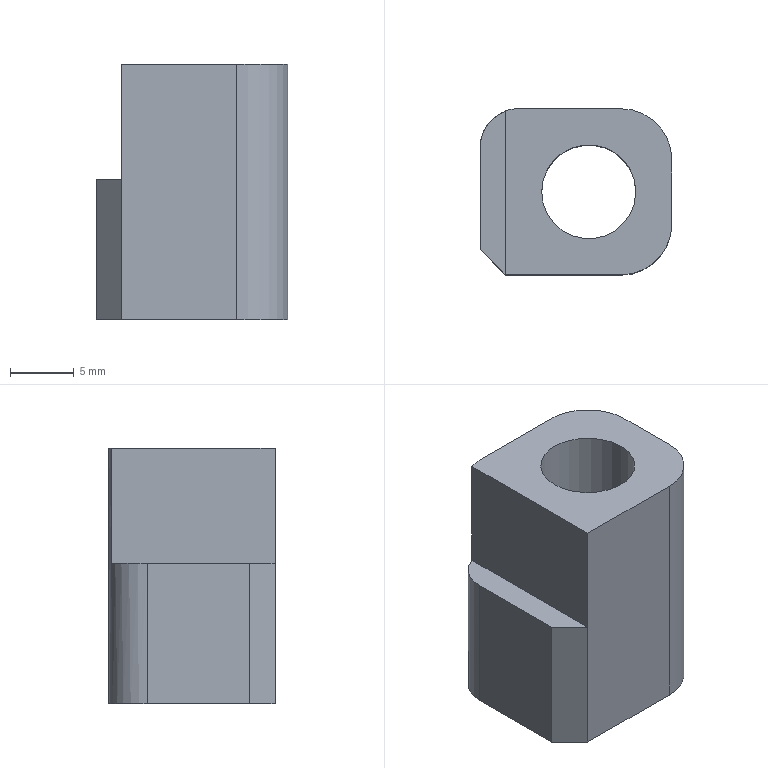Part | STEP file | 1 solid | 13 faces | box 15 x 13 x 20 mm | volume 2634 mm3 | plane 9 | cylinder 4 | commonest cylinder face diameters 8 x2 6 x1 7.36 x1
STEP:
#1=CARTESIAN_POINT('',(272.5,-10.,-2.));
#2=VERTEX_POINT('',#1);
#3=CARTESIAN_POINT('',(272.5,-15.,-2.));
#4=VERTEX_POINT('',#3);
#5=CARTESIAN_POINT('',(272.5,-12.5,-2.));
#6=DIRECTION('',(0.,-1.,0.));
#7=VECTOR('',#6,1.);
#8=LINE('',#5,#7);
#9=EDGE_CURVE('',#2,#4,#8,.T.);
#10=ORIENTED_EDGE('',*,*,#9,.F.);
#11=CARTESIAN_POINT('',(268.5,-6.,-2.));
#12=VERTEX_POINT('',#11);
#13=CARTESIAN_POINT('',(268.5,-10.,-2.));
#14=DIRECTION('',(0.,0.,1.));
#15=DIRECTION('',(1.,0.,0.));
#16=AXIS2_PLACEMENT_3D('',#13,#14,#15);
#17=CIRCLE('',#16,4.);
#18=EDGE_CURVE('',#2,#12,#17,.T.);
#19=ORIENTED_EDGE('',*,*,#18,.T.);
#20=CARTESIAN_POINT('',(260.5,-6.,-2.));
#21=VERTEX_POINT('',#20);
#22=CARTESIAN_POINT('',(266.,-6.,-2.));
#23=DIRECTION('',(1.,0.,0.));
#24=VECTOR('',#23,1.);
#25=LINE('',#22,#24);
#26=EDGE_CURVE('',#21,#12,#25,.T.);
#27=ORIENTED_EDGE('',*,*,#26,.F.);
#28=CARTESIAN_POINT('',(259.5,-6.172,-2.));
#29=VERTEX_POINT('',#28);
#30=CARTESIAN_POINT('',(260.5,-9.,-2.));
#31=DIRECTION('',(0.,0.,1.));
#32=DIRECTION('',(1.,0.,0.));
#33=AXIS2_PLACEMENT_3D('',#30,#31,#32);
#34=CIRCLE('',#33,3.);
#35=EDGE_CURVE('',#21,#29,#34,.T.);
#36=ORIENTED_EDGE('',*,*,#35,.T.);
#37=CARTESIAN_POINT('',(259.5,-19.,-2.));
#38=VERTEX_POINT('',#37);
#39=CARTESIAN_POINT('',(259.5,-12.5,-2.));
#40=DIRECTION('',(0.,1.,0.));
#41=VECTOR('',#40,1.);
#42=LINE('',#39,#41);
#43=EDGE_CURVE('',#38,#29,#42,.T.);
#44=ORIENTED_EDGE('',*,*,#43,.F.);
#45=CARTESIAN_POINT('',(268.5,-19.,-2.));
#46=VERTEX_POINT('',#45);
#47=CARTESIAN_POINT('',(266.,-19.,-2.));
#48=DIRECTION('',(-1.,0.,0.));
#49=VECTOR('',#48,1.);
#50=LINE('',#47,#49);
#51=EDGE_CURVE('',#46,#38,#50,.T.);
#52=ORIENTED_EDGE('',*,*,#51,.F.);
#53=CARTESIAN_POINT('',(268.5,-15.,-2.));
#54=DIRECTION('',(0.,0.,1.));
#55=DIRECTION('',(1.,0.,0.));
#56=AXIS2_PLACEMENT_3D('',#53,#54,#55);
#57=CIRCLE('',#56,4.);
#58=EDGE_CURVE('',#46,#4,#57,.T.);
#59=ORIENTED_EDGE('',*,*,#58,.T.);
#60=EDGE_LOOP('',(#10,#19,#27,#36,#44,#52,#59));
#61=FACE_BOUND('',#60,.T.);
#62=CARTESIAN_POINT('',(269.68,-12.5,-2.));
#63=VERTEX_POINT('',#62);
#64=CARTESIAN_POINT('',(266.,-12.5,-2.));
#65=DIRECTION('',(0.,0.,-1.));
#66=DIRECTION('',(1.,0.,0.));
#67=AXIS2_PLACEMENT_3D('',#64,#65,#66);
#68=CIRCLE('',#67,3.68);
#69=EDGE_CURVE('',#63,#63,#68,.T.);
#70=ORIENTED_EDGE('',*,*,#69,.T.);
#71=EDGE_LOOP('',(#70));
#72=FACE_BOUND('',#71,.T.);
#73=CARTESIAN_POINT('',(266.,-12.5,-2.));
#74=DIRECTION('',(0.,0.,1.));
#75=DIRECTION('',(1.,0.,0.));
#76=AXIS2_PLACEMENT_3D('',#73,#74,#75);
#77=PLANE('',#76);
#78=ADVANCED_FACE('',(#61,#72),#77,.T.);
#79=CARTESIAN_POINT('',(259.5,-19.,-11.));
#80=VERTEX_POINT('',#79);
#81=CARTESIAN_POINT('',(259.5,-19.,-22.));
#82=DIRECTION('',(0.,0.,1.));
#83=VECTOR('',#82,1.);
#84=LINE('',#81,#83);
#85=EDGE_CURVE('',#80,#38,#84,.T.);
#86=ORIENTED_EDGE('',*,*,#85,.F.);
#87=CARTESIAN_POINT('',(259.5,-19.,-22.));
#88=VERTEX_POINT('',#87);
#89=CARTESIAN_POINT('',(259.5,-19.,-22.));
#90=DIRECTION('',(0.,0.,-1.));
#91=VECTOR('',#90,1.);
#92=LINE('',#89,#91);
#93=EDGE_CURVE('',#80,#88,#92,.T.);
#94=ORIENTED_EDGE('',*,*,#93,.T.);
#95=CARTESIAN_POINT('',(268.5,-19.,-22.));
#96=VERTEX_POINT('',#95);
#97=CARTESIAN_POINT('',(266.,-19.,-22.));
#98=DIRECTION('',(1.,0.,0.));
#99=VECTOR('',#98,1.);
#100=LINE('',#97,#99);
#101=EDGE_CURVE('',#88,#96,#100,.T.);
#102=ORIENTED_EDGE('',*,*,#101,.T.);
#103=CARTESIAN_POINT('',(268.5,-19.,-22.));
#104=DIRECTION('',(0.,0.,1.));
#105=VECTOR('',#104,1.);
#106=LINE('',#103,#105);
#107=EDGE_CURVE('',#96,#46,#106,.T.);
#108=ORIENTED_EDGE('',*,*,#107,.T.);
#109=ORIENTED_EDGE('',*,*,#51,.T.);
#110=EDGE_LOOP('',(#86,#94,#102,#108,#109));
#111=FACE_OUTER_BOUND('',#110,.T.);
#112=CARTESIAN_POINT('',(266.,-19.,-22.));
#113=DIRECTION('',(0.,-1.,0.));
#114=DIRECTION('',(0.,0.,-1.));
#115=AXIS2_PLACEMENT_3D('',#112,#113,#114);
#116=PLANE('',#115);
#117=ADVANCED_FACE('',(#111),#116,.T.);
#118=ORIENTED_EDGE('',*,*,#43,.T.);
#119=CARTESIAN_POINT('',(259.5,-6.172,-11.));
#120=VERTEX_POINT('',#119);
#121=CARTESIAN_POINT('',(259.5,-6.172,-2.));
#122=DIRECTION('',(0.,0.,-1.));
#123=VECTOR('',#122,1.);
#124=LINE('',#121,#123);
#125=EDGE_CURVE('',#29,#120,#124,.T.);
#126=ORIENTED_EDGE('',*,*,#125,.T.);
#127=CARTESIAN_POINT('',(259.5,-12.5,-11.));
#128=DIRECTION('',(0.,1.,0.));
#129=VECTOR('',#128,1.);
#130=LINE('',#127,#129);
#131=EDGE_CURVE('',#80,#120,#130,.T.);
#132=ORIENTED_EDGE('',*,*,#131,.F.);
#133=ORIENTED_EDGE('',*,*,#85,.T.);
#134=EDGE_LOOP('',(#118,#126,#132,#133));
#135=FACE_OUTER_BOUND('',#134,.T.);
#136=CARTESIAN_POINT('',(259.5,-12.5,-22.));
#137=DIRECTION('',(-1.,0.,0.));
#138=DIRECTION('',(0.,0.,1.));
#139=AXIS2_PLACEMENT_3D('',#136,#137,#138);
#140=PLANE('',#139);
#141=ADVANCED_FACE('',(#135),#140,.T.);
#142=ORIENTED_EDGE('',*,*,#26,.T.);
#143=CARTESIAN_POINT('',(268.5,-6.,-22.));
#144=VERTEX_POINT('',#143);
#145=CARTESIAN_POINT('',(268.5,-6.,-22.));
#146=DIRECTION('',(0.,0.,-1.));
#147=VECTOR('',#146,1.);
#148=LINE('',#145,#147);
#149=EDGE_CURVE('',#12,#144,#148,.T.);
#150=ORIENTED_EDGE('',*,*,#149,.T.);
#151=CARTESIAN_POINT('',(260.5,-6.,-22.));
#152=VERTEX_POINT('',#151);
#153=CARTESIAN_POINT('',(266.,-6.,-22.));
#154=DIRECTION('',(-1.,0.,0.));
#155=VECTOR('',#154,1.);
#156=LINE('',#153,#155);
#157=EDGE_CURVE('',#144,#152,#156,.T.);
#158=ORIENTED_EDGE('',*,*,#157,.T.);
#159=CARTESIAN_POINT('',(260.5,-6.,-22.));
#160=DIRECTION('',(0.,0.,1.));
#161=VECTOR('',#160,1.);
#162=LINE('',#159,#161);
#163=EDGE_CURVE('',#152,#21,#162,.T.);
#164=ORIENTED_EDGE('',*,*,#163,.T.);
#165=EDGE_LOOP('',(#142,#150,#158,#164));
#166=FACE_OUTER_BOUND('',#165,.T.);
#167=CARTESIAN_POINT('',(266.,-6.,-22.));
#168=DIRECTION('',(0.,1.,0.));
#169=DIRECTION('',(0.,0.,1.));
#170=AXIS2_PLACEMENT_3D('',#167,#168,#169);
#171=PLANE('',#170);
#172=ADVANCED_FACE('',(#166),#171,.T.);
#173=ORIENTED_EDGE('',*,*,#101,.F.);
#174=CARTESIAN_POINT('',(257.5,-17.,-22.));
#175=VERTEX_POINT('',#174);
#176=CARTESIAN_POINT('',(259.5,-19.,-22.));
#177=DIRECTION('',(-0.7071,0.7071,0.));
#178=VECTOR('',#177,1.);
#179=LINE('',#176,#178);
#180=EDGE_CURVE('',#88,#175,#179,.T.);
#181=ORIENTED_EDGE('',*,*,#180,.T.);
#182=CARTESIAN_POINT('',(257.5,-9.,-22.));
#183=VERTEX_POINT('',#182);
#184=CARTESIAN_POINT('',(257.5,-12.5,-22.));
#185=DIRECTION('',(0.,-1.,0.));
#186=VECTOR('',#185,1.);
#187=LINE('',#184,#186);
#188=EDGE_CURVE('',#183,#175,#187,.T.);
#189=ORIENTED_EDGE('',*,*,#188,.F.);
#190=CARTESIAN_POINT('',(260.5,-9.,-22.));
#191=DIRECTION('',(0.,0.,-1.));
#192=DIRECTION('',(-1.,0.,0.));
#193=AXIS2_PLACEMENT_3D('',#190,#191,#192);
#194=CIRCLE('',#193,3.);
#195=EDGE_CURVE('',#183,#152,#194,.T.);
#196=ORIENTED_EDGE('',*,*,#195,.T.);
#197=ORIENTED_EDGE('',*,*,#157,.F.);
#198=CARTESIAN_POINT('',(272.5,-10.,-22.));
#199=VERTEX_POINT('',#198);
#200=CARTESIAN_POINT('',(268.5,-10.,-22.));
#201=DIRECTION('',(0.,0.,-1.));
#202=DIRECTION('',(-1.,0.,0.));
#203=AXIS2_PLACEMENT_3D('',#200,#201,#202);
#204=CIRCLE('',#203,4.);
#205=EDGE_CURVE('',#144,#199,#204,.T.);
#206=ORIENTED_EDGE('',*,*,#205,.T.);
#207=CARTESIAN_POINT('',(272.5,-15.,-22.));
#208=VERTEX_POINT('',#207);
#209=CARTESIAN_POINT('',(272.5,-12.5,-22.));
#210=DIRECTION('',(0.,1.,0.));
#211=VECTOR('',#210,1.);
#212=LINE('',#209,#211);
#213=EDGE_CURVE('',#208,#199,#212,.T.);
#214=ORIENTED_EDGE('',*,*,#213,.F.);
#215=CARTESIAN_POINT('',(268.5,-15.,-22.));
#216=DIRECTION('',(0.,0.,-1.));
#217=DIRECTION('',(-1.,0.,0.));
#218=AXIS2_PLACEMENT_3D('',#215,#216,#217);
#219=CIRCLE('',#218,4.);
#220=EDGE_CURVE('',#208,#96,#219,.T.);
#221=ORIENTED_EDGE('',*,*,#220,.T.);
#222=EDGE_LOOP('',(#173,#181,#189,#196,#197,#206,#214,#221));
#223=FACE_BOUND('',#222,.T.);
#224=CARTESIAN_POINT('',(262.32,-12.5,-22.));
#225=VERTEX_POINT('',#224);
#226=CARTESIAN_POINT('',(266.,-12.5,-22.));
#227=DIRECTION('',(0.,0.,-1.));
#228=DIRECTION('',(-1.,0.,0.));
#229=AXIS2_PLACEMENT_3D('',#226,#227,#228);
#230=CIRCLE('',#229,3.68);
#231=EDGE_CURVE('',#225,#225,#230,.T.);
#232=ORIENTED_EDGE('',*,*,#231,.F.);
#233=EDGE_LOOP('',(#232));
#234=FACE_BOUND('',#233,.T.);
#235=CARTESIAN_POINT('',(266.,-12.5,-22.));
#236=DIRECTION('',(0.,0.,-1.));
#237=DIRECTION('',(-1.,0.,0.));
#238=AXIS2_PLACEMENT_3D('',#235,#236,#237);
#239=PLANE('',#238);
#240=ADVANCED_FACE('',(#223,#234),#239,.T.);
#241=ORIENTED_EDGE('',*,*,#213,.T.);
#242=CARTESIAN_POINT('',(272.5,-10.,-22.));
#243=DIRECTION('',(0.,0.,1.));
#244=VECTOR('',#243,1.);
#245=LINE('',#242,#244);
#246=EDGE_CURVE('',#199,#2,#245,.T.);
#247=ORIENTED_EDGE('',*,*,#246,.T.);
#248=ORIENTED_EDGE('',*,*,#9,.T.);
#249=CARTESIAN_POINT('',(272.5,-15.,-22.));
#250=DIRECTION('',(0.,0.,-1.));
#251=VECTOR('',#250,1.);
#252=LINE('',#249,#251);
#253=EDGE_CURVE('',#4,#208,#252,.T.);
#254=ORIENTED_EDGE('',*,*,#253,.T.);
#255=EDGE_LOOP('',(#241,#247,#248,#254));
#256=FACE_OUTER_BOUND('',#255,.T.);
#257=CARTESIAN_POINT('',(272.5,-12.5,-22.));
#258=DIRECTION('',(1.,0.,0.));
#259=DIRECTION('',(0.,0.,-1.));
#260=AXIS2_PLACEMENT_3D('',#257,#258,#259);
#261=PLANE('',#260);
#262=ADVANCED_FACE('',(#256),#261,.T.);
#263=ORIENTED_EDGE('',*,*,#69,.F.);
#264=EDGE_LOOP('',(#263));
#265=FACE_BOUND('',#264,.T.);
#266=ORIENTED_EDGE('',*,*,#231,.T.);
#267=EDGE_LOOP('',(#266));
#268=FACE_BOUND('',#267,.T.);
#269=CARTESIAN_POINT('',(266.,-12.5,-75.));
#270=DIRECTION('',(0.,0.,1.));
#271=DIRECTION('',(1.,0.,0.));
#272=AXIS2_PLACEMENT_3D('',#269,#270,#271);
#273=CYLINDRICAL_SURFACE('',#272,3.68);
#274=ADVANCED_FACE('',(#265,#268),#273,.F.);
#275=CARTESIAN_POINT('',(257.5,-17.,-11.));
#276=VERTEX_POINT('',#275);
#277=CARTESIAN_POINT('',(257.5,-9.,-11.));
#278=VERTEX_POINT('',#277);
#279=CARTESIAN_POINT('',(257.5,-12.5,-11.));
#280=DIRECTION('',(0.,1.,0.));
#281=VECTOR('',#280,1.);
#282=LINE('',#279,#281);
#283=EDGE_CURVE('',#276,#278,#282,.T.);
#284=ORIENTED_EDGE('',*,*,#283,.F.);
#285=CARTESIAN_POINT('',(257.5,-17.,-11.));
#286=DIRECTION('',(0.7071,-0.7071,0.));
#287=VECTOR('',#286,1.);
#288=LINE('',#285,#287);
#289=EDGE_CURVE('',#276,#80,#288,.T.);
#290=ORIENTED_EDGE('',*,*,#289,.T.);
#291=ORIENTED_EDGE('',*,*,#131,.T.);
#292=CARTESIAN_POINT('',(260.5,-9.,-11.));
#293=DIRECTION('',(0.,0.,1.));
#294=DIRECTION('',(1.,0.,0.));
#295=AXIS2_PLACEMENT_3D('',#292,#293,#294);
#296=CIRCLE('',#295,3.);
#297=EDGE_CURVE('',#120,#278,#296,.T.);
#298=ORIENTED_EDGE('',*,*,#297,.T.);
#299=EDGE_LOOP('',(#284,#290,#291,#298));
#300=FACE_OUTER_BOUND('',#299,.T.);
#301=CARTESIAN_POINT('',(259.5,-12.5,-11.));
#302=DIRECTION('',(0.,0.,1.));
#303=DIRECTION('',(0.,1.,0.));
#304=AXIS2_PLACEMENT_3D('',#301,#302,#303);
#305=PLANE('',#304);
#306=ADVANCED_FACE('',(#300),#305,.T.);
#307=ORIENTED_EDGE('',*,*,#188,.T.);
#308=CARTESIAN_POINT('',(257.5,-17.,-22.));
#309=DIRECTION('',(0.,0.,1.));
#310=VECTOR('',#309,1.);
#311=LINE('',#308,#310);
#312=EDGE_CURVE('',#175,#276,#311,.T.);
#313=ORIENTED_EDGE('',*,*,#312,.T.);
#314=ORIENTED_EDGE('',*,*,#283,.T.);
#315=CARTESIAN_POINT('',(257.5,-9.,-22.));
#316=DIRECTION('',(0.,0.,-1.));
#317=VECTOR('',#316,1.);
#318=LINE('',#315,#317);
#319=EDGE_CURVE('',#278,#183,#318,.T.);
#320=ORIENTED_EDGE('',*,*,#319,.T.);
#321=EDGE_LOOP('',(#307,#313,#314,#320));
#322=FACE_OUTER_BOUND('',#321,.T.);
#323=CARTESIAN_POINT('',(257.5,-12.5,-22.));
#324=DIRECTION('',(-1.,0.,0.));
#325=DIRECTION('',(0.,0.,1.));
#326=AXIS2_PLACEMENT_3D('',#323,#324,#325);
#327=PLANE('',#326);
#328=ADVANCED_FACE('',(#322),#327,.T.);
#329=ORIENTED_EDGE('',*,*,#195,.F.);
#330=ORIENTED_EDGE('',*,*,#319,.F.);
#331=ORIENTED_EDGE('',*,*,#297,.F.);
#332=ORIENTED_EDGE('',*,*,#125,.F.);
#333=ORIENTED_EDGE('',*,*,#35,.F.);
#334=ORIENTED_EDGE('',*,*,#163,.F.);
#335=EDGE_LOOP('',(#329,#330,#331,#332,#333,#334));
#336=FACE_OUTER_BOUND('',#335,.T.);
#337=CARTESIAN_POINT('',(260.5,-9.,-22.));
#338=DIRECTION('',(0.,0.,1.));
#339=DIRECTION('',(1.,0.,0.));
#340=AXIS2_PLACEMENT_3D('',#337,#338,#339);
#341=CYLINDRICAL_SURFACE('',#340,3.);
#342=ADVANCED_FACE('',(#336),#341,.T.);
#343=ORIENTED_EDGE('',*,*,#205,.F.);
#344=ORIENTED_EDGE('',*,*,#149,.F.);
#345=ORIENTED_EDGE('',*,*,#18,.F.);
#346=ORIENTED_EDGE('',*,*,#246,.F.);
#347=EDGE_LOOP('',(#343,#344,#345,#346));
#348=FACE_OUTER_BOUND('',#347,.T.);
#349=CARTESIAN_POINT('',(268.5,-10.,-22.));
#350=DIRECTION('',(0.,0.,1.));
#351=DIRECTION('',(1.,0.,0.));
#352=AXIS2_PLACEMENT_3D('',#349,#350,#351);
#353=CYLINDRICAL_SURFACE('',#352,4.);
#354=ADVANCED_FACE('',(#348),#353,.T.);
#355=ORIENTED_EDGE('',*,*,#220,.F.);
#356=ORIENTED_EDGE('',*,*,#253,.F.);
#357=ORIENTED_EDGE('',*,*,#58,.F.);
#358=ORIENTED_EDGE('',*,*,#107,.F.);
#359=EDGE_LOOP('',(#355,#356,#357,#358));
#360=FACE_OUTER_BOUND('',#359,.T.);
#361=CARTESIAN_POINT('',(268.5,-15.,-22.));
#362=DIRECTION('',(0.,0.,1.));
#363=DIRECTION('',(1.,0.,0.));
#364=AXIS2_PLACEMENT_3D('',#361,#362,#363);
#365=CYLINDRICAL_SURFACE('',#364,4.);
#366=ADVANCED_FACE('',(#360),#365,.T.);
#367=ORIENTED_EDGE('',*,*,#180,.F.);
#368=ORIENTED_EDGE('',*,*,#93,.F.);
#369=ORIENTED_EDGE('',*,*,#289,.F.);
#370=ORIENTED_EDGE('',*,*,#312,.F.);
#371=EDGE_LOOP('',(#367,#368,#369,#370));
#372=FACE_OUTER_BOUND('',#371,.T.);
#373=CARTESIAN_POINT('',(257.5,-17.,-22.));
#374=DIRECTION('',(0.7071,0.7071,0.));
#375=DIRECTION('',(0.,0.,1.));
#376=AXIS2_PLACEMENT_3D('',#373,#374,#375);
#377=PLANE('',#376);
#378=ADVANCED_FACE('',(#372),#377,.F.);
#379=CLOSED_SHELL('',(#78,#117,#141,#172,#240,#262,#274,#306,#328,#342,#354,#366,#378));
#380=MANIFOLD_SOLID_BREP('',#379);
#381=(LENGTH_UNIT()NAMED_UNIT(*)SI_UNIT(.MILLI.,.METRE.));
#382=UNCERTAINTY_MEASURE_WITH_UNIT(LENGTH_MEASURE(0.00002),#381,'','');
#383=(NAMED_UNIT(*)PLANE_ANGLE_UNIT()SI_UNIT($,.RADIAN.));
#384=PLANE_ANGLE_MEASURE_WITH_UNIT(PLANE_ANGLE_MEASURE(0.01745),#383);
#385=DIMENSIONAL_EXPONENTS(0.,0.,0.,0.,0.,0.,0.);
#386=(CONVERSION_BASED_UNIT('DEGREE',#384)NAMED_UNIT(#385)PLANE_ANGLE_UNIT());
#387=(NAMED_UNIT(*)SI_UNIT($,.STERADIAN.)SOLID_ANGLE_UNIT());
#388=(GEOMETRIC_REPRESENTATION_CONTEXT(3)GLOBAL_UNCERTAINTY_ASSIGNED_CONTEXT((#382))GLOBAL_UNIT_ASSIGNED_CONTEXT((#381,#386,#387))REPRESENTATION_CONTEXT('',''));
#389=ADVANCED_BREP_SHAPE_REPRESENTATION('',(#380),#388);